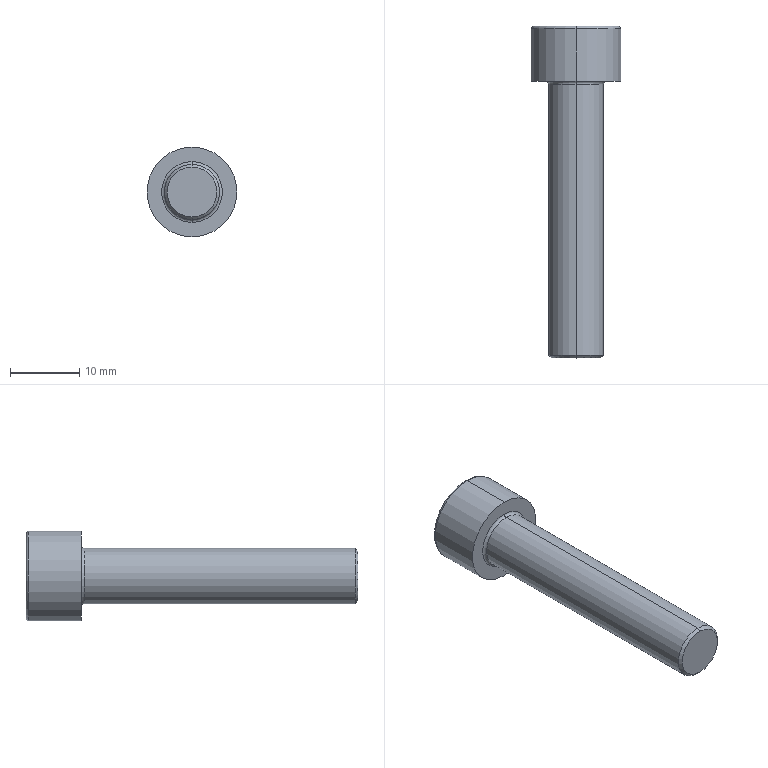Part | STEP file | 1 solid | 20 faces | box 13 x 48 x 13 mm | volume 2945 mm3 | plane 10 | torus 4 | cylinder 4 | cone 2 | commonest cylinder face diameters 8 x2 13 x2
STEP:
#1=CARTESIAN_POINT('',(0.,-40.,-3.6));
#2=VERTEX_POINT('',#1);
#3=CARTESIAN_POINT('',(0.,-40.,3.6));
#4=VERTEX_POINT('',#3);
#5=CARTESIAN_POINT('',(0.,-40.,0.));
#6=DIRECTION('',(0.,-1.,0.));
#7=DIRECTION('',(0.,0.,-1.));
#8=AXIS2_PLACEMENT_3D('',#5,#6,#7);
#9=CIRCLE('',#8,3.6);
#10=EDGE_CURVE('',#2,#4,#9,.T.);
#11=ORIENTED_EDGE('',*,*,#10,.F.);
#12=CARTESIAN_POINT('',(0.,-39.6,-4.));
#13=VERTEX_POINT('',#12);
#14=CARTESIAN_POINT('',(0.,-40.,-3.6));
#15=DIRECTION('',(0.,0.7071,-0.7071));
#16=VECTOR('',#15,1000.);
#17=LINE('',#14,#16);
#18=EDGE_CURVE('',#2,#13,#17,.T.);
#19=ORIENTED_EDGE('',*,*,#18,.T.);
#20=CARTESIAN_POINT('',(0.,-39.6,4.));
#21=VERTEX_POINT('',#20);
#22=CARTESIAN_POINT('',(0.,-39.6,0.));
#23=DIRECTION('',(0.,1.,0.));
#24=DIRECTION('',(0.,0.,-1.));
#25=AXIS2_PLACEMENT_3D('',#22,#23,#24);
#26=CIRCLE('',#25,4.);
#27=EDGE_CURVE('',#21,#13,#26,.T.);
#28=ORIENTED_EDGE('',*,*,#27,.F.);
#29=CARTESIAN_POINT('',(0.,-40.,3.6));
#30=DIRECTION('',(0.,0.7071,0.7071));
#31=VECTOR('',#30,1000.);
#32=LINE('',#29,#31);
#33=EDGE_CURVE('',#4,#21,#32,.T.);
#34=ORIENTED_EDGE('',*,*,#33,.F.);
#35=EDGE_LOOP('',(#11,#19,#28,#34));
#36=FACE_OUTER_BOUND('',#35,.T.);
#37=CARTESIAN_POINT('',(0.,-40.,0.));
#38=DIRECTION('',(0.,1.,0.));
#39=DIRECTION('',(0.,0.,1.));
#40=AXIS2_PLACEMENT_3D('',#37,#38,#39);
#41=CONICAL_SURFACE('',#40,3.6,0.7854);
#42=ADVANCED_FACE('',(#36),#41,.T.);
#43=CARTESIAN_POINT('',(0.,7.6,-6.5));
#44=VERTEX_POINT('',#43);
#45=CARTESIAN_POINT('',(0.,7.6,6.5));
#46=VERTEX_POINT('',#45);
#47=CARTESIAN_POINT('',(0.,7.6,0.));
#48=DIRECTION('',(0.,-1.,0.));
#49=DIRECTION('',(0.,0.,1.));
#50=AXIS2_PLACEMENT_3D('',#47,#48,#49);
#51=CIRCLE('',#50,6.5);
#52=EDGE_CURVE('',#44,#46,#51,.T.);
#53=ORIENTED_EDGE('',*,*,#52,.F.);
#54=CARTESIAN_POINT('',(0.,8.,-6.1));
#55=VERTEX_POINT('',#54);
#56=CARTESIAN_POINT('',(0.,7.6,-6.1));
#57=DIRECTION('',(1.,0.,0.));
#58=DIRECTION('',(0.,0.,-1.));
#59=AXIS2_PLACEMENT_3D('',#56,#57,#58);
#60=CIRCLE('',#59,0.4);
#61=EDGE_CURVE('',#44,#55,#60,.T.);
#62=ORIENTED_EDGE('',*,*,#61,.T.);
#63=CARTESIAN_POINT('',(0.,8.,6.1));
#64=VERTEX_POINT('',#63);
#65=CARTESIAN_POINT('',(0.,8.,0.));
#66=DIRECTION('',(0.,1.,0.));
#67=DIRECTION('',(0.,0.,1.));
#68=AXIS2_PLACEMENT_3D('',#65,#66,#67);
#69=CIRCLE('',#68,6.1);
#70=EDGE_CURVE('',#64,#55,#69,.T.);
#71=ORIENTED_EDGE('',*,*,#70,.F.);
#72=CARTESIAN_POINT('',(0.,7.6,6.1));
#73=DIRECTION('',(-1.,0.,0.));
#74=DIRECTION('',(0.,0.,1.));
#75=AXIS2_PLACEMENT_3D('',#72,#73,#74);
#76=CIRCLE('',#75,0.4);
#77=EDGE_CURVE('',#46,#64,#76,.T.);
#78=ORIENTED_EDGE('',*,*,#77,.F.);
#79=EDGE_LOOP('',(#53,#62,#71,#78));
#80=FACE_OUTER_BOUND('',#79,.T.);
#81=CARTESIAN_POINT('',(0.,7.6,0.));
#82=DIRECTION('',(0.,1.,0.));
#83=DIRECTION('',(0.,0.,1.));
#84=AXIS2_PLACEMENT_3D('',#81,#82,#83);
#85=TOROIDAL_SURFACE('',#84,6.1,0.4);
#86=ADVANCED_FACE('',(#80),#85,.T.);
#87=CARTESIAN_POINT('',(0.,-0.4,4.));
#88=VERTEX_POINT('',#87);
#89=CARTESIAN_POINT('',(0.,-0.4,-4.));
#90=VERTEX_POINT('',#89);
#91=CARTESIAN_POINT('',(0.,-0.4,0.));
#92=DIRECTION('',(0.,-1.,0.));
#93=DIRECTION('',(0.,0.,-1.));
#94=AXIS2_PLACEMENT_3D('',#91,#92,#93);
#95=CIRCLE('',#94,4.);
#96=EDGE_CURVE('',#88,#90,#95,.T.);
#97=ORIENTED_EDGE('',*,*,#96,.F.);
#98=CARTESIAN_POINT('',(0.,0.,4.4));
#99=VERTEX_POINT('',#98);
#100=CARTESIAN_POINT('',(0.,-0.4,4.4));
#101=DIRECTION('',(1.,0.,0.));
#102=DIRECTION('',(0.,0.,-1.));
#103=AXIS2_PLACEMENT_3D('',#100,#101,#102);
#104=CIRCLE('',#103,0.4);
#105=EDGE_CURVE('',#88,#99,#104,.T.);
#106=ORIENTED_EDGE('',*,*,#105,.T.);
#107=CARTESIAN_POINT('',(0.,0.,-4.4));
#108=VERTEX_POINT('',#107);
#109=CARTESIAN_POINT('',(0.,0.,0.));
#110=DIRECTION('',(0.,1.,0.));
#111=DIRECTION('',(0.,0.,-1.));
#112=AXIS2_PLACEMENT_3D('',#109,#110,#111);
#113=CIRCLE('',#112,4.4);
#114=EDGE_CURVE('',#108,#99,#113,.T.);
#115=ORIENTED_EDGE('',*,*,#114,.F.);
#116=CARTESIAN_POINT('',(0.,-0.4,-4.4));
#117=DIRECTION('',(-1.,0.,0.));
#118=DIRECTION('',(0.,0.,1.));
#119=AXIS2_PLACEMENT_3D('',#116,#117,#118);
#120=CIRCLE('',#119,0.4);
#121=EDGE_CURVE('',#90,#108,#120,.T.);
#122=ORIENTED_EDGE('',*,*,#121,.F.);
#123=EDGE_LOOP('',(#97,#106,#115,#122));
#124=FACE_OUTER_BOUND('',#123,.T.);
#125=CARTESIAN_POINT('',(0.,-0.4,0.));
#126=DIRECTION('',(0.,-1.,0.));
#127=DIRECTION('',(0.,0.,-1.));
#128=AXIS2_PLACEMENT_3D('',#125,#126,#127);
#129=TOROIDAL_SURFACE('',#128,4.4,0.4);
#130=ADVANCED_FACE('',(#124),#129,.F.);
#131=CARTESIAN_POINT('',(0.,-0.4,0.));
#132=DIRECTION('',(0.,-1.,0.));
#133=DIRECTION('',(0.,0.,-1.));
#134=AXIS2_PLACEMENT_3D('',#131,#132,#133);
#135=CIRCLE('',#134,4.);
#136=EDGE_CURVE('',#90,#88,#135,.T.);
#137=ORIENTED_EDGE('',*,*,#136,.T.);
#138=CARTESIAN_POINT('',(0.,0.,4.));
#139=DIRECTION('',(0.,-1.,0.));
#140=VECTOR('',#139,1000.);
#141=LINE('',#138,#140);
#142=EDGE_CURVE('',#88,#21,#141,.T.);
#143=ORIENTED_EDGE('',*,*,#142,.T.);
#144=ORIENTED_EDGE('',*,*,#27,.T.);
#145=CARTESIAN_POINT('',(0.,0.,-4.));
#146=DIRECTION('',(0.,-1.,0.));
#147=VECTOR('',#146,1000.);
#148=LINE('',#145,#147);
#149=EDGE_CURVE('',#90,#13,#148,.T.);
#150=ORIENTED_EDGE('',*,*,#149,.F.);
#151=EDGE_LOOP('',(#137,#143,#144,#150));
#152=FACE_OUTER_BOUND('',#151,.T.);
#153=CARTESIAN_POINT('',(0.,0.,0.));
#154=DIRECTION('',(0.,-1.,0.));
#155=DIRECTION('',(0.,0.,-1.));
#156=AXIS2_PLACEMENT_3D('',#153,#154,#155);
#157=CYLINDRICAL_SURFACE('',#156,4.);
#158=ADVANCED_FACE('',(#152),#157,.T.);
#159=ORIENTED_EDGE('',*,*,#52,.T.);
#160=CARTESIAN_POINT('',(0.,0.,6.5));
#161=VERTEX_POINT('',#160);
#162=CARTESIAN_POINT('',(0.,0.,6.5));
#163=DIRECTION('',(0.,-1.,0.));
#164=VECTOR('',#163,1000.);
#165=LINE('',#162,#164);
#166=EDGE_CURVE('',#46,#161,#165,.T.);
#167=ORIENTED_EDGE('',*,*,#166,.T.);
#168=CARTESIAN_POINT('',(0.,0.,-6.5));
#169=VERTEX_POINT('',#168);
#170=CARTESIAN_POINT('',(0.,0.,0.));
#171=DIRECTION('',(0.,-1.,0.));
#172=DIRECTION('',(0.,0.,-1.));
#173=AXIS2_PLACEMENT_3D('',#170,#171,#172);
#174=CIRCLE('',#173,6.5);
#175=EDGE_CURVE('',#169,#161,#174,.T.);
#176=ORIENTED_EDGE('',*,*,#175,.F.);
#177=CARTESIAN_POINT('',(0.,0.,-6.5));
#178=DIRECTION('',(0.,-1.,0.));
#179=VECTOR('',#178,1000.);
#180=LINE('',#177,#179);
#181=EDGE_CURVE('',#44,#169,#180,.T.);
#182=ORIENTED_EDGE('',*,*,#181,.F.);
#183=EDGE_LOOP('',(#159,#167,#176,#182));
#184=FACE_OUTER_BOUND('',#183,.T.);
#185=CARTESIAN_POINT('',(0.,0.,0.));
#186=DIRECTION('',(0.,-1.,0.));
#187=DIRECTION('',(0.,0.,-1.));
#188=AXIS2_PLACEMENT_3D('',#185,#186,#187);
#189=CYLINDRICAL_SURFACE('',#188,6.5);
#190=ADVANCED_FACE('',(#184),#189,.T.);
#191=ORIENTED_EDGE('',*,*,#70,.T.);
#192=CARTESIAN_POINT('',(0.,8.,0.));
#193=DIRECTION('',(0.,1.,0.));
#194=DIRECTION('',(0.,0.,1.));
#195=AXIS2_PLACEMENT_3D('',#192,#193,#194);
#196=CIRCLE('',#195,6.1);
#197=EDGE_CURVE('',#55,#64,#196,.T.);
#198=ORIENTED_EDGE('',*,*,#197,.T.);
#199=EDGE_LOOP('',(#191,#198));
#200=FACE_OUTER_BOUND('',#199,.T.);
#201=CARTESIAN_POINT('',(0.,8.,-3.464));
#202=VERTEX_POINT('',#201);
#203=CARTESIAN_POINT('',(-3.,8.,-1.732));
#204=VERTEX_POINT('',#203);
#205=CARTESIAN_POINT('',(0.,8.,-3.464));
#206=DIRECTION('',(-0.866,0.,0.5));
#207=VECTOR('',#206,1000.);
#208=LINE('',#205,#207);
#209=EDGE_CURVE('',#202,#204,#208,.T.);
#210=ORIENTED_EDGE('',*,*,#209,.F.);
#211=CARTESIAN_POINT('',(3.,8.,-1.732));
#212=VERTEX_POINT('',#211);
#213=CARTESIAN_POINT('',(3.,8.,-1.732));
#214=DIRECTION('',(-0.866,0.,-0.5));
#215=VECTOR('',#214,1000.);
#216=LINE('',#213,#215);
#217=EDGE_CURVE('',#212,#202,#216,.T.);
#218=ORIENTED_EDGE('',*,*,#217,.F.);
#219=CARTESIAN_POINT('',(3.,8.,1.732));
#220=VERTEX_POINT('',#219);
#221=CARTESIAN_POINT('',(3.,8.,1.732));
#222=DIRECTION('',(0.,0.,-1.));
#223=VECTOR('',#222,1000.);
#224=LINE('',#221,#223);
#225=EDGE_CURVE('',#220,#212,#224,.T.);
#226=ORIENTED_EDGE('',*,*,#225,.F.);
#227=CARTESIAN_POINT('',(0.,8.,3.464));
#228=VERTEX_POINT('',#227);
#229=CARTESIAN_POINT('',(0.,8.,3.464));
#230=DIRECTION('',(0.866,0.,-0.5));
#231=VECTOR('',#230,1000.);
#232=LINE('',#229,#231);
#233=EDGE_CURVE('',#228,#220,#232,.T.);
#234=ORIENTED_EDGE('',*,*,#233,.F.);
#235=CARTESIAN_POINT('',(-3.,8.,1.732));
#236=VERTEX_POINT('',#235);
#237=CARTESIAN_POINT('',(-3.,8.,1.732));
#238=DIRECTION('',(0.866,0.,0.5));
#239=VECTOR('',#238,1000.);
#240=LINE('',#237,#239);
#241=EDGE_CURVE('',#236,#228,#240,.T.);
#242=ORIENTED_EDGE('',*,*,#241,.F.);
#243=CARTESIAN_POINT('',(-3.,8.,-1.732));
#244=DIRECTION('',(0.,0.,1.));
#245=VECTOR('',#244,1000.);
#246=LINE('',#243,#245);
#247=EDGE_CURVE('',#204,#236,#246,.T.);
#248=ORIENTED_EDGE('',*,*,#247,.F.);
#249=EDGE_LOOP('',(#210,#218,#226,#234,#242,#248));
#250=FACE_BOUND('',#249,.T.);
#251=CARTESIAN_POINT('',(0.,8.,0.));
#252=DIRECTION('',(0.,1.,0.));
#253=DIRECTION('',(0.,0.,1.));
#254=AXIS2_PLACEMENT_3D('',#251,#252,#253);
#255=PLANE('',#254);
#256=ADVANCED_FACE('',(#200,#250),#255,.T.);
#257=ORIENTED_EDGE('',*,*,#166,.F.);
#258=CARTESIAN_POINT('',(0.,7.6,0.));
#259=DIRECTION('',(0.,-1.,0.));
#260=DIRECTION('',(0.,0.,1.));
#261=AXIS2_PLACEMENT_3D('',#258,#259,#260);
#262=CIRCLE('',#261,6.5);
#263=EDGE_CURVE('',#46,#44,#262,.T.);
#264=ORIENTED_EDGE('',*,*,#263,.T.);
#265=ORIENTED_EDGE('',*,*,#181,.T.);
#266=CARTESIAN_POINT('',(0.,0.,0.));
#267=DIRECTION('',(0.,-1.,0.));
#268=DIRECTION('',(0.,0.,-1.));
#269=AXIS2_PLACEMENT_3D('',#266,#267,#268);
#270=CIRCLE('',#269,6.5);
#271=EDGE_CURVE('',#161,#169,#270,.T.);
#272=ORIENTED_EDGE('',*,*,#271,.F.);
#273=EDGE_LOOP('',(#257,#264,#265,#272));
#274=FACE_OUTER_BOUND('',#273,.T.);
#275=CARTESIAN_POINT('',(0.,0.,0.));
#276=DIRECTION('',(0.,-1.,0.));
#277=DIRECTION('',(0.,0.,-1.));
#278=AXIS2_PLACEMENT_3D('',#275,#276,#277);
#279=CYLINDRICAL_SURFACE('',#278,6.5);
#280=ADVANCED_FACE('',(#274),#279,.T.);
#281=ORIENTED_EDGE('',*,*,#114,.T.);
#282=CARTESIAN_POINT('',(0.,0.,0.));
#283=DIRECTION('',(0.,1.,0.));
#284=DIRECTION('',(0.,0.,-1.));
#285=AXIS2_PLACEMENT_3D('',#282,#283,#284);
#286=CIRCLE('',#285,4.4);
#287=EDGE_CURVE('',#99,#108,#286,.T.);
#288=ORIENTED_EDGE('',*,*,#287,.T.);
#289=EDGE_LOOP('',(#281,#288));
#290=FACE_BOUND('',#289,.T.);
#291=ORIENTED_EDGE('',*,*,#175,.T.);
#292=ORIENTED_EDGE('',*,*,#271,.T.);
#293=EDGE_LOOP('',(#291,#292));
#294=FACE_OUTER_BOUND('',#293,.T.);
#295=CARTESIAN_POINT('',(6.5,0.,0.));
#296=DIRECTION('',(0.,-1.,0.));
#297=DIRECTION('',(0.,0.,-1.));
#298=AXIS2_PLACEMENT_3D('',#295,#296,#297);
#299=PLANE('',#298);
#300=ADVANCED_FACE('',(#290,#294),#299,.T.);
#301=ORIENTED_EDGE('',*,*,#142,.F.);
#302=ORIENTED_EDGE('',*,*,#96,.T.);
#303=ORIENTED_EDGE('',*,*,#149,.T.);
#304=CARTESIAN_POINT('',(0.,-39.6,0.));
#305=DIRECTION('',(0.,1.,0.));
#306=DIRECTION('',(0.,0.,-1.));
#307=AXIS2_PLACEMENT_3D('',#304,#305,#306);
#308=CIRCLE('',#307,4.);
#309=EDGE_CURVE('',#13,#21,#308,.T.);
#310=ORIENTED_EDGE('',*,*,#309,.T.);
#311=EDGE_LOOP('',(#301,#302,#303,#310));
#312=FACE_OUTER_BOUND('',#311,.T.);
#313=CARTESIAN_POINT('',(0.,0.,0.));
#314=DIRECTION('',(0.,-1.,0.));
#315=DIRECTION('',(0.,0.,-1.));
#316=AXIS2_PLACEMENT_3D('',#313,#314,#315);
#317=CYLINDRICAL_SURFACE('',#316,4.);
#318=ADVANCED_FACE('',(#312),#317,.T.);
#319=CARTESIAN_POINT('',(0.,-40.,0.));
#320=DIRECTION('',(0.,-1.,0.));
#321=DIRECTION('',(0.,0.,-1.));
#322=AXIS2_PLACEMENT_3D('',#319,#320,#321);
#323=CIRCLE('',#322,3.6);
#324=EDGE_CURVE('',#4,#2,#323,.T.);
#325=ORIENTED_EDGE('',*,*,#324,.T.);
#326=ORIENTED_EDGE('',*,*,#10,.T.);
#327=EDGE_LOOP('',(#325,#326));
#328=FACE_OUTER_BOUND('',#327,.T.);
#329=CARTESIAN_POINT('',(4.,-40.,0.));
#330=DIRECTION('',(0.,-1.,0.));
#331=DIRECTION('',(0.,0.,-1.));
#332=AXIS2_PLACEMENT_3D('',#329,#330,#331);
#333=PLANE('',#332);
#334=ADVANCED_FACE('',(#328),#333,.T.);
#335=ORIENTED_EDGE('',*,*,#209,.T.);
#336=CARTESIAN_POINT('',(-3.,4.,-1.732));
#337=VERTEX_POINT('',#336);
#338=CARTESIAN_POINT('',(-3.,4.,-1.732));
#339=DIRECTION('',(0.,1.,0.));
#340=VECTOR('',#339,1000.);
#341=LINE('',#338,#340);
#342=EDGE_CURVE('',#337,#204,#341,.T.);
#343=ORIENTED_EDGE('',*,*,#342,.F.);
#344=CARTESIAN_POINT('',(0.,4.,-3.464));
#345=VERTEX_POINT('',#344);
#346=CARTESIAN_POINT('',(0.,4.,-3.464));
#347=DIRECTION('',(-0.866,0.,0.5));
#348=VECTOR('',#347,1000.);
#349=LINE('',#346,#348);
#350=EDGE_CURVE('',#345,#337,#349,.T.);
#351=ORIENTED_EDGE('',*,*,#350,.F.);
#352=CARTESIAN_POINT('',(0.,4.,-3.464));
#353=DIRECTION('',(0.,1.,0.));
#354=VECTOR('',#353,1000.);
#355=LINE('',#352,#354);
#356=EDGE_CURVE('',#345,#202,#355,.T.);
#357=ORIENTED_EDGE('',*,*,#356,.T.);
#358=EDGE_LOOP('',(#335,#343,#351,#357));
#359=FACE_OUTER_BOUND('',#358,.T.);
#360=CARTESIAN_POINT('',(0.,4.,-3.464));
#361=DIRECTION('',(-0.5,0.,-0.866));
#362=DIRECTION('',(-0.866,0.,0.5));
#363=AXIS2_PLACEMENT_3D('',#360,#361,#362);
#364=PLANE('',#363);
#365=ADVANCED_FACE('',(#359),#364,.F.);
#366=ORIENTED_EDGE('',*,*,#217,.T.);
#367=ORIENTED_EDGE('',*,*,#356,.F.);
#368=CARTESIAN_POINT('',(3.,4.,-1.732));
#369=VERTEX_POINT('',#368);
#370=CARTESIAN_POINT('',(3.,4.,-1.732));
#371=DIRECTION('',(-0.866,0.,-0.5));
#372=VECTOR('',#371,1000.);
#373=LINE('',#370,#372);
#374=EDGE_CURVE('',#369,#345,#373,.T.);
#375=ORIENTED_EDGE('',*,*,#374,.F.);
#376=CARTESIAN_POINT('',(3.,4.,-1.732));
#377=DIRECTION('',(0.,1.,0.));
#378=VECTOR('',#377,1000.);
#379=LINE('',#376,#378);
#380=EDGE_CURVE('',#369,#212,#379,.T.);
#381=ORIENTED_EDGE('',*,*,#380,.T.);
#382=EDGE_LOOP('',(#366,#367,#375,#381));
#383=FACE_OUTER_BOUND('',#382,.T.);
#384=CARTESIAN_POINT('',(3.,4.,-1.732));
#385=DIRECTION('',(0.5,0.,-0.866));
#386=DIRECTION('',(-0.866,0.,-0.5));
#387=AXIS2_PLACEMENT_3D('',#384,#385,#386);
#388=PLANE('',#387);
#389=ADVANCED_FACE('',(#383),#388,.F.);
#390=ORIENTED_EDGE('',*,*,#225,.T.);
#391=ORIENTED_EDGE('',*,*,#380,.F.);
#392=CARTESIAN_POINT('',(3.,4.,1.732));
#393=VERTEX_POINT('',#392);
#394=CARTESIAN_POINT('',(3.,4.,1.732));
#395=DIRECTION('',(0.,0.,-1.));
#396=VECTOR('',#395,1000.);
#397=LINE('',#394,#396);
#398=EDGE_CURVE('',#393,#369,#397,.T.);
#399=ORIENTED_EDGE('',*,*,#398,.F.);
#400=CARTESIAN_POINT('',(3.,4.,1.732));
#401=DIRECTION('',(0.,1.,0.));
#402=VECTOR('',#401,1000.);
#403=LINE('',#400,#402);
#404=EDGE_CURVE('',#393,#220,#403,.T.);
#405=ORIENTED_EDGE('',*,*,#404,.T.);
#406=EDGE_LOOP('',(#390,#391,#399,#405));
#407=FACE_OUTER_BOUND('',#406,.T.);
#408=CARTESIAN_POINT('',(3.,4.,1.732));
#409=DIRECTION('',(1.,0.,0.));
#410=DIRECTION('',(0.,0.,-1.));
#411=AXIS2_PLACEMENT_3D('',#408,#409,#410);
#412=PLANE('',#411);
#413=ADVANCED_FACE('',(#407),#412,.F.);
#414=ORIENTED_EDGE('',*,*,#233,.T.);
#415=ORIENTED_EDGE('',*,*,#404,.F.);
#416=CARTESIAN_POINT('',(0.,4.,3.464));
#417=VERTEX_POINT('',#416);
#418=CARTESIAN_POINT('',(0.,4.,3.464));
#419=DIRECTION('',(0.866,0.,-0.5));
#420=VECTOR('',#419,1000.);
#421=LINE('',#418,#420);
#422=EDGE_CURVE('',#417,#393,#421,.T.);
#423=ORIENTED_EDGE('',*,*,#422,.F.);
#424=CARTESIAN_POINT('',(0.,4.,3.464));
#425=DIRECTION('',(0.,1.,0.));
#426=VECTOR('',#425,1000.);
#427=LINE('',#424,#426);
#428=EDGE_CURVE('',#417,#228,#427,.T.);
#429=ORIENTED_EDGE('',*,*,#428,.T.);
#430=EDGE_LOOP('',(#414,#415,#423,#429));
#431=FACE_OUTER_BOUND('',#430,.T.);
#432=CARTESIAN_POINT('',(0.,4.,3.464));
#433=DIRECTION('',(0.5,0.,0.866));
#434=DIRECTION('',(0.866,0.,-0.5));
#435=AXIS2_PLACEMENT_3D('',#432,#433,#434);
#436=PLANE('',#435);
#437=ADVANCED_FACE('',(#431),#436,.F.);
#438=ORIENTED_EDGE('',*,*,#241,.T.);
#439=ORIENTED_EDGE('',*,*,#428,.F.);
#440=CARTESIAN_POINT('',(-3.,4.,1.732));
#441=VERTEX_POINT('',#440);
#442=CARTESIAN_POINT('',(-3.,4.,1.732));
#443=DIRECTION('',(0.866,0.,0.5));
#444=VECTOR('',#443,1000.);
#445=LINE('',#442,#444);
#446=EDGE_CURVE('',#441,#417,#445,.T.);
#447=ORIENTED_EDGE('',*,*,#446,.F.);
#448=CARTESIAN_POINT('',(-3.,4.,1.732));
#449=DIRECTION('',(0.,1.,0.));
#450=VECTOR('',#449,1000.);
#451=LINE('',#448,#450);
#452=EDGE_CURVE('',#441,#236,#451,.T.);
#453=ORIENTED_EDGE('',*,*,#452,.T.);
#454=EDGE_LOOP('',(#438,#439,#447,#453));
#455=FACE_OUTER_BOUND('',#454,.T.);
#456=CARTESIAN_POINT('',(-3.,4.,1.732));
#457=DIRECTION('',(-0.5,0.,0.866));
#458=DIRECTION('',(0.866,0.,0.5));
#459=AXIS2_PLACEMENT_3D('',#456,#457,#458);
#460=PLANE('',#459);
#461=ADVANCED_FACE('',(#455),#460,.F.);
#462=ORIENTED_EDGE('',*,*,#247,.T.);
#463=ORIENTED_EDGE('',*,*,#452,.F.);
#464=CARTESIAN_POINT('',(-3.,4.,-1.732));
#465=DIRECTION('',(0.,0.,1.));
#466=VECTOR('',#465,1000.);
#467=LINE('',#464,#466);
#468=EDGE_CURVE('',#337,#441,#467,.T.);
#469=ORIENTED_EDGE('',*,*,#468,.F.);
#470=ORIENTED_EDGE('',*,*,#342,.T.);
#471=EDGE_LOOP('',(#462,#463,#469,#470));
#472=FACE_OUTER_BOUND('',#471,.T.);
#473=CARTESIAN_POINT('',(-3.,4.,-1.732));
#474=DIRECTION('',(-1.,0.,0.));
#475=DIRECTION('',(0.,0.,1.));
#476=AXIS2_PLACEMENT_3D('',#473,#474,#475);
#477=PLANE('',#476);
#478=ADVANCED_FACE('',(#472),#477,.F.);
#479=ORIENTED_EDGE('',*,*,#350,.T.);
#480=ORIENTED_EDGE('',*,*,#468,.T.);
#481=ORIENTED_EDGE('',*,*,#446,.T.);
#482=ORIENTED_EDGE('',*,*,#422,.T.);
#483=ORIENTED_EDGE('',*,*,#398,.T.);
#484=ORIENTED_EDGE('',*,*,#374,.T.);
#485=EDGE_LOOP('',(#479,#480,#481,#482,#483,#484));
#486=FACE_OUTER_BOUND('',#485,.T.);
#487=CARTESIAN_POINT('',(0.,4.,0.));
#488=DIRECTION('',(0.,1.,0.));
#489=DIRECTION('',(0.,0.,1.));
#490=AXIS2_PLACEMENT_3D('',#487,#488,#489);
#491=PLANE('',#490);
#492=ADVANCED_FACE('',(#486),#491,.T.);
#493=ORIENTED_EDGE('',*,*,#105,.F.);
#494=ORIENTED_EDGE('',*,*,#136,.F.);
#495=ORIENTED_EDGE('',*,*,#121,.T.);
#496=ORIENTED_EDGE('',*,*,#287,.F.);
#497=EDGE_LOOP('',(#493,#494,#495,#496));
#498=FACE_OUTER_BOUND('',#497,.T.);
#499=CARTESIAN_POINT('',(0.,-0.4,0.));
#500=DIRECTION('',(0.,-1.,0.));
#501=DIRECTION('',(0.,0.,-1.));
#502=AXIS2_PLACEMENT_3D('',#499,#500,#501);
#503=TOROIDAL_SURFACE('',#502,4.4,0.4);
#504=ADVANCED_FACE('',(#498),#503,.F.);
#505=ORIENTED_EDGE('',*,*,#61,.F.);
#506=ORIENTED_EDGE('',*,*,#263,.F.);
#507=ORIENTED_EDGE('',*,*,#77,.T.);
#508=ORIENTED_EDGE('',*,*,#197,.F.);
#509=EDGE_LOOP('',(#505,#506,#507,#508));
#510=FACE_OUTER_BOUND('',#509,.T.);
#511=CARTESIAN_POINT('',(0.,7.6,0.));
#512=DIRECTION('',(0.,1.,0.));
#513=DIRECTION('',(0.,0.,1.));
#514=AXIS2_PLACEMENT_3D('',#511,#512,#513);
#515=TOROIDAL_SURFACE('',#514,6.1,0.4);
#516=ADVANCED_FACE('',(#510),#515,.T.);
#517=ORIENTED_EDGE('',*,*,#18,.F.);
#518=ORIENTED_EDGE('',*,*,#324,.F.);
#519=ORIENTED_EDGE('',*,*,#33,.T.);
#520=ORIENTED_EDGE('',*,*,#309,.F.);
#521=EDGE_LOOP('',(#517,#518,#519,#520));
#522=FACE_OUTER_BOUND('',#521,.T.);
#523=CARTESIAN_POINT('',(0.,-40.,0.));
#524=DIRECTION('',(0.,1.,0.));
#525=DIRECTION('',(0.,0.,1.));
#526=AXIS2_PLACEMENT_3D('',#523,#524,#525);
#527=CONICAL_SURFACE('',#526,3.6,0.7854);
#528=ADVANCED_FACE('',(#522),#527,.T.);
#529=CLOSED_SHELL('',(#42,#86,#130,#158,#190,#256,#280,#300,#318,#334,#365,#389,#413,#437,#461,#478,#492,#504,#516,#528));
#530=MANIFOLD_SOLID_BREP('',#529);
#531=CARTESIAN_POINT('',(0.,0.,0.));
#532=DIRECTION('',(0.,0.,1.));
#533=DIRECTION('',(1.,0.,0.));
#534=AXIS2_PLACEMENT_3D('',#531,#532,#533);
#535=(LENGTH_UNIT()NAMED_UNIT(*)SI_UNIT(.MILLI.,.METRE.));
#536=UNCERTAINTY_MEASURE_WITH_UNIT(LENGTH_MEASURE(0.00001),#535,'','');
#537=(NAMED_UNIT(*)PLANE_ANGLE_UNIT()SI_UNIT($,.RADIAN.));
#538=(NAMED_UNIT(*)SI_UNIT($,.STERADIAN.)SOLID_ANGLE_UNIT());
#539=(GEOMETRIC_REPRESENTATION_CONTEXT(3)GLOBAL_UNCERTAINTY_ASSIGNED_CONTEXT((#536))GLOBAL_UNIT_ASSIGNED_CONTEXT((#535,#537,#538))REPRESENTATION_CONTEXT('',''));
#540=ADVANCED_BREP_SHAPE_REPRESENTATION('',(#530,#534),#539);